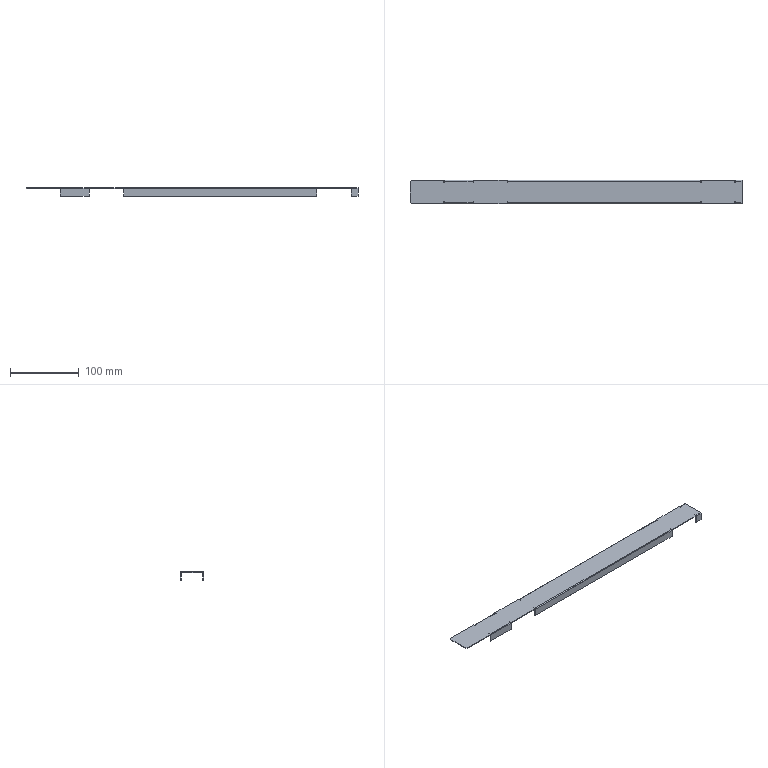Part | SolidWorks | features SMBaseFlange 2, Chamfer 1, Cut 1, EdgeFlange 1, FlatPattern 1, ICE 1, MirrorPattern 1, SheetMetal 1 | 1 solid | 96 faces | box 483.5 x 34 x 12 mm | volume 23557 mm3 | plane 84 | cylinder 12 | commonest cylinder face diameters 0.4 x6 2.4 x6